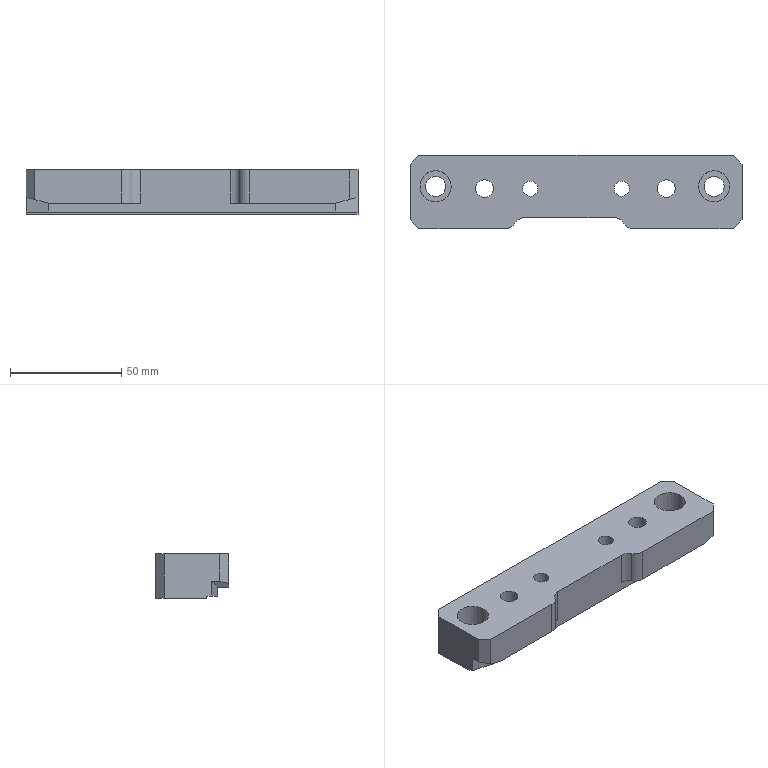Part | NX | features 20 2 | 1 solid | 34 faces | box 149 x 33 x 20 mm | volume 81598 mm3 | plane 22 | cylinder 12 | commonest cylinder face diameters 10 x4 6.8 x2 8.001 x2 9 x2 14 x2
STEP:
#1=CARTESIAN_POINT('',(540.502,427.372,-3.5));
#2=VERTEX_POINT('',#1);
#3=CARTESIAN_POINT('',(540.502,427.372,-2.5));
#4=VERTEX_POINT('',#3);
#5=CARTESIAN_POINT('',(540.502,427.372,11.5));
#6=DIRECTION('',(0.,0.,1.));
#7=VECTOR('',#6,1000.);
#8=LINE('',#5,#7);
#9=EDGE_CURVE('',#2,#4,#8,.T.);
#10=ORIENTED_EDGE('',*,*,#9,.F.);
#11=CARTESIAN_POINT('',(540.502,446.5,-3.5));
#12=VERTEX_POINT('',#11);
#13=CARTESIAN_POINT('',(540.502,450.5,-3.5));
#14=DIRECTION('',(0.,1.,0.));
#15=VECTOR('',#14,1000.);
#16=LINE('',#13,#15);
#17=EDGE_CURVE('',#2,#12,#16,.T.);
#18=ORIENTED_EDGE('',*,*,#17,.T.);
#19=CARTESIAN_POINT('',(540.502,446.5,16.5));
#20=VERTEX_POINT('',#19);
#21=CARTESIAN_POINT('',(540.502,446.5,11.5));
#22=DIRECTION('',(0.,0.,1.));
#23=VECTOR('',#22,1000.);
#24=LINE('',#21,#23);
#25=EDGE_CURVE('',#12,#20,#24,.T.);
#26=ORIENTED_EDGE('',*,*,#25,.T.);
#27=CARTESIAN_POINT('',(540.502,421.5,16.5));
#28=VERTEX_POINT('',#27);
#29=CARTESIAN_POINT('',(540.502,450.5,16.5));
#30=DIRECTION('',(0.,1.,0.));
#31=VECTOR('',#30,1000.);
#32=LINE('',#29,#31);
#33=EDGE_CURVE('',#28,#20,#32,.T.);
#34=ORIENTED_EDGE('',*,*,#33,.F.);
#35=CARTESIAN_POINT('',(540.502,421.5,4.179));
#36=VERTEX_POINT('',#35);
#37=CARTESIAN_POINT('',(540.502,421.5,11.5));
#38=DIRECTION('',(0.,0.,-1.));
#39=VECTOR('',#38,1000.);
#40=LINE('',#37,#39);
#41=EDGE_CURVE('',#28,#36,#40,.T.);
#42=ORIENTED_EDGE('',*,*,#41,.T.);
#43=CARTESIAN_POINT('',(540.502,425.18,4.179));
#44=VERTEX_POINT('',#43);
#45=CARTESIAN_POINT('',(540.502,417.5,4.179));
#46=DIRECTION('',(0.,1.,0.));
#47=VECTOR('',#46,1000.);
#48=LINE('',#45,#47);
#49=EDGE_CURVE('',#36,#44,#48,.T.);
#50=ORIENTED_EDGE('',*,*,#49,.T.);
#51=CARTESIAN_POINT('',(540.502,425.18,-2.5));
#52=VERTEX_POINT('',#51);
#53=CARTESIAN_POINT('',(540.502,425.18,3.5));
#54=DIRECTION('',(0.,0.,1.));
#55=VECTOR('',#54,1000.);
#56=LINE('',#53,#55);
#57=EDGE_CURVE('',#52,#44,#56,.T.);
#58=ORIENTED_EDGE('',*,*,#57,.F.);
#59=CARTESIAN_POINT('',(540.502,450.5,-2.5));
#60=DIRECTION('',(0.,1.,0.));
#61=VECTOR('',#60,1000.);
#62=LINE('',#59,#61);
#63=EDGE_CURVE('',#52,#4,#62,.T.);
#64=ORIENTED_EDGE('',*,*,#63,.T.);
#65=EDGE_LOOP('',(#10,#18,#26,#34,#42,#50,#58,#64));
#66=FACE_BOUND('',#65,.T.);
#67=CARTESIAN_POINT('',(540.502,450.5,11.5));
#68=DIRECTION('',(-1.,0.,0.));
#69=DIRECTION('',(0.,0.,-1.));
#70=AXIS2_PLACEMENT_3D('',#67,#68,#69);
#71=PLANE('',#70);
#72=ADVANCED_FACE('',(#66),#71,.F.);
#73=CARTESIAN_POINT('',(391.502,427.372,-2.5));
#74=VERTEX_POINT('',#73);
#75=CARTESIAN_POINT('',(391.502,427.372,-3.5));
#76=VERTEX_POINT('',#75);
#77=CARTESIAN_POINT('',(391.502,427.372,11.5));
#78=DIRECTION('',(0.,0.,-1.));
#79=VECTOR('',#78,1000.);
#80=LINE('',#77,#79);
#81=EDGE_CURVE('',#74,#76,#80,.T.);
#82=ORIENTED_EDGE('',*,*,#81,.F.);
#83=CARTESIAN_POINT('',(391.502,425.179,-2.5));
#84=VERTEX_POINT('',#83);
#85=CARTESIAN_POINT('',(391.502,417.5,-2.5));
#86=DIRECTION('',(0.,-1.,0.));
#87=VECTOR('',#86,1000.);
#88=LINE('',#85,#87);
#89=EDGE_CURVE('',#74,#84,#88,.T.);
#90=ORIENTED_EDGE('',*,*,#89,.T.);
#91=CARTESIAN_POINT('',(391.502,425.179,4.179));
#92=VERTEX_POINT('',#91);
#93=CARTESIAN_POINT('',(391.502,425.179,3.5));
#94=DIRECTION('',(0.,0.,1.));
#95=VECTOR('',#94,1000.);
#96=LINE('',#93,#95);
#97=EDGE_CURVE('',#84,#92,#96,.T.);
#98=ORIENTED_EDGE('',*,*,#97,.T.);
#99=CARTESIAN_POINT('',(391.502,421.5,4.179));
#100=VERTEX_POINT('',#99);
#101=CARTESIAN_POINT('',(391.502,425.179,4.179));
#102=DIRECTION('',(0.,-1.,0.));
#103=VECTOR('',#102,1000.);
#104=LINE('',#101,#103);
#105=EDGE_CURVE('',#92,#100,#104,.T.);
#106=ORIENTED_EDGE('',*,*,#105,.T.);
#107=CARTESIAN_POINT('',(391.502,421.5,16.5));
#108=VERTEX_POINT('',#107);
#109=CARTESIAN_POINT('',(391.502,421.5,11.5));
#110=DIRECTION('',(0.,0.,1.));
#111=VECTOR('',#110,1000.);
#112=LINE('',#109,#111);
#113=EDGE_CURVE('',#100,#108,#112,.T.);
#114=ORIENTED_EDGE('',*,*,#113,.T.);
#115=CARTESIAN_POINT('',(391.502,446.5,16.5));
#116=VERTEX_POINT('',#115);
#117=CARTESIAN_POINT('',(391.502,417.5,16.5));
#118=DIRECTION('',(0.,-1.,0.));
#119=VECTOR('',#118,1000.);
#120=LINE('',#117,#119);
#121=EDGE_CURVE('',#116,#108,#120,.T.);
#122=ORIENTED_EDGE('',*,*,#121,.F.);
#123=CARTESIAN_POINT('',(391.502,446.5,-3.5));
#124=VERTEX_POINT('',#123);
#125=CARTESIAN_POINT('',(391.502,446.5,11.5));
#126=DIRECTION('',(0.,0.,-1.));
#127=VECTOR('',#126,1000.);
#128=LINE('',#125,#127);
#129=EDGE_CURVE('',#116,#124,#128,.T.);
#130=ORIENTED_EDGE('',*,*,#129,.T.);
#131=CARTESIAN_POINT('',(391.502,417.5,-3.5));
#132=DIRECTION('',(0.,-1.,0.));
#133=VECTOR('',#132,1000.);
#134=LINE('',#131,#133);
#135=EDGE_CURVE('',#124,#76,#134,.T.);
#136=ORIENTED_EDGE('',*,*,#135,.T.);
#137=EDGE_LOOP('',(#82,#90,#98,#106,#114,#122,#130,#136));
#138=FACE_BOUND('',#137,.T.);
#139=CARTESIAN_POINT('',(391.502,417.5,11.5));
#140=DIRECTION('',(1.,0.,0.));
#141=DIRECTION('',(0.,0.,1.));
#142=AXIS2_PLACEMENT_3D('',#139,#140,#141);
#143=PLANE('',#142);
#144=ADVANCED_FACE('',(#138),#143,.F.);
#145=CARTESIAN_POINT('',(429.002,435.5,16.5));
#146=VERTEX_POINT('',#145);
#147=CARTESIAN_POINT('',(425.002,435.5,16.5));
#148=DIRECTION('',(0.,0.,1.));
#149=DIRECTION('',(1.,0.,0.));
#150=AXIS2_PLACEMENT_3D('',#147,#148,#149);
#151=CIRCLE('',#150,4.);
#152=EDGE_CURVE('',#146,#146,#151,.T.);
#153=ORIENTED_EDGE('',*,*,#152,.F.);
#154=EDGE_LOOP('',(#153));
#155=FACE_BOUND('',#154,.T.);
#156=CARTESIAN_POINT('',(510.502,435.5,16.5));
#157=VERTEX_POINT('',#156);
#158=CARTESIAN_POINT('',(506.502,435.5,16.5));
#159=DIRECTION('',(0.,0.,1.));
#160=DIRECTION('',(1.,0.,0.));
#161=AXIS2_PLACEMENT_3D('',#158,#159,#160);
#162=CIRCLE('',#161,4.);
#163=EDGE_CURVE('',#157,#157,#162,.T.);
#164=ORIENTED_EDGE('',*,*,#163,.F.);
#165=EDGE_LOOP('',(#164));
#166=FACE_BOUND('',#165,.T.);
#167=CARTESIAN_POINT('',(410.002,436.5,16.5));
#168=VERTEX_POINT('',#167);
#169=CARTESIAN_POINT('',(403.002,436.5,16.5));
#170=DIRECTION('',(0.,0.,1.));
#171=DIRECTION('',(1.,0.,0.));
#172=AXIS2_PLACEMENT_3D('',#169,#170,#171);
#173=CIRCLE('',#172,7.);
#174=EDGE_CURVE('',#168,#168,#173,.T.);
#175=ORIENTED_EDGE('',*,*,#174,.F.);
#176=EDGE_LOOP('',(#175));
#177=FACE_BOUND('',#176,.T.);
#178=CARTESIAN_POINT('',(535.002,436.5,16.5));
#179=VERTEX_POINT('',#178);
#180=CARTESIAN_POINT('',(528.002,436.5,16.5));
#181=DIRECTION('',(0.,0.,-1.));
#182=DIRECTION('',(1.,0.,0.));
#183=AXIS2_PLACEMENT_3D('',#180,#181,#182);
#184=CIRCLE('',#183,7.);
#185=EDGE_CURVE('',#179,#179,#184,.T.);
#186=ORIENTED_EDGE('',*,*,#185,.T.);
#187=EDGE_LOOP('',(#186));
#188=FACE_BOUND('',#187,.T.);
#189=ORIENTED_EDGE('',*,*,#121,.T.);
#190=CARTESIAN_POINT('',(395.502,417.5,16.5));
#191=VERTEX_POINT('',#190);
#192=CARTESIAN_POINT('',(391.502,421.5,16.5));
#193=DIRECTION('',(0.7071,-0.7071,0.));
#194=VECTOR('',#193,1000.);
#195=LINE('',#192,#194);
#196=EDGE_CURVE('',#108,#191,#195,.T.);
#197=ORIENTED_EDGE('',*,*,#196,.T.);
#198=CARTESIAN_POINT('',(434.268,417.5,16.5));
#199=VERTEX_POINT('',#198);
#200=CARTESIAN_POINT('',(368.002,417.5,16.5));
#201=DIRECTION('',(1.,0.,0.));
#202=VECTOR('',#201,1000.);
#203=LINE('',#200,#202);
#204=EDGE_CURVE('',#191,#199,#203,.T.);
#205=ORIENTED_EDGE('',*,*,#204,.T.);
#206=CARTESIAN_POINT('',(438.598,420.,16.5));
#207=VERTEX_POINT('',#206);
#208=CARTESIAN_POINT('',(434.268,422.5,16.5));
#209=DIRECTION('',(0.,0.,1.));
#210=DIRECTION('',(1.,0.,0.));
#211=AXIS2_PLACEMENT_3D('',#208,#209,#210);
#212=CIRCLE('',#211,5.);
#213=EDGE_CURVE('',#199,#207,#212,.T.);
#214=ORIENTED_EDGE('',*,*,#213,.T.);
#215=CARTESIAN_POINT('',(442.929,422.5,16.5));
#216=VERTEX_POINT('',#215);
#217=CARTESIAN_POINT('',(442.929,417.5,16.5));
#218=DIRECTION('',(0.,0.,1.));
#219=DIRECTION('',(1.,0.,0.));
#220=AXIS2_PLACEMENT_3D('',#217,#218,#219);
#221=CIRCLE('',#220,5.);
#222=EDGE_CURVE('',#216,#207,#221,.T.);
#223=ORIENTED_EDGE('',*,*,#222,.F.);
#224=CARTESIAN_POINT('',(483.129,422.5,16.5));
#225=VERTEX_POINT('',#224);
#226=CARTESIAN_POINT('',(368.002,422.5,16.5));
#227=DIRECTION('',(-1.,0.,0.));
#228=VECTOR('',#227,1000.);
#229=LINE('',#226,#228);
#230=EDGE_CURVE('',#225,#216,#229,.T.);
#231=ORIENTED_EDGE('',*,*,#230,.F.);
#232=CARTESIAN_POINT('',(487.459,420.,16.5));
#233=VERTEX_POINT('',#232);
#234=CARTESIAN_POINT('',(483.129,417.5,16.5));
#235=DIRECTION('',(0.,0.,1.));
#236=DIRECTION('',(1.,0.,0.));
#237=AXIS2_PLACEMENT_3D('',#234,#235,#236);
#238=CIRCLE('',#237,5.);
#239=EDGE_CURVE('',#233,#225,#238,.T.);
#240=ORIENTED_EDGE('',*,*,#239,.F.);
#241=CARTESIAN_POINT('',(491.789,417.5,16.5));
#242=VERTEX_POINT('',#241);
#243=CARTESIAN_POINT('',(491.789,422.5,16.5));
#244=DIRECTION('',(0.,0.,1.));
#245=DIRECTION('',(1.,0.,0.));
#246=AXIS2_PLACEMENT_3D('',#243,#244,#245);
#247=CIRCLE('',#246,5.);
#248=EDGE_CURVE('',#233,#242,#247,.T.);
#249=ORIENTED_EDGE('',*,*,#248,.T.);
#250=CARTESIAN_POINT('',(536.502,417.5,16.5));
#251=VERTEX_POINT('',#250);
#252=CARTESIAN_POINT('',(368.002,417.5,16.5));
#253=DIRECTION('',(1.,0.,0.));
#254=VECTOR('',#253,1000.);
#255=LINE('',#252,#254);
#256=EDGE_CURVE('',#242,#251,#255,.T.);
#257=ORIENTED_EDGE('',*,*,#256,.T.);
#258=CARTESIAN_POINT('',(536.502,417.5,16.5));
#259=DIRECTION('',(0.7071,0.7071,0.));
#260=VECTOR('',#259,1000.);
#261=LINE('',#258,#260);
#262=EDGE_CURVE('',#251,#28,#261,.T.);
#263=ORIENTED_EDGE('',*,*,#262,.T.);
#264=ORIENTED_EDGE('',*,*,#33,.T.);
#265=CARTESIAN_POINT('',(536.502,450.5,16.5));
#266=VERTEX_POINT('',#265);
#267=CARTESIAN_POINT('',(540.502,446.5,16.5));
#268=DIRECTION('',(-0.7071,0.7071,0.));
#269=VECTOR('',#268,1000.);
#270=LINE('',#267,#269);
#271=EDGE_CURVE('',#20,#266,#270,.T.);
#272=ORIENTED_EDGE('',*,*,#271,.T.);
#273=CARTESIAN_POINT('',(395.502,450.5,16.5));
#274=VERTEX_POINT('',#273);
#275=CARTESIAN_POINT('',(288.002,450.5,16.5));
#276=DIRECTION('',(-1.,0.,0.));
#277=VECTOR('',#276,1000.);
#278=LINE('',#275,#277);
#279=EDGE_CURVE('',#266,#274,#278,.T.);
#280=ORIENTED_EDGE('',*,*,#279,.T.);
#281=CARTESIAN_POINT('',(395.502,450.5,16.5));
#282=DIRECTION('',(-0.7071,-0.7071,0.));
#283=VECTOR('',#282,1000.);
#284=LINE('',#281,#283);
#285=EDGE_CURVE('',#274,#116,#284,.T.);
#286=ORIENTED_EDGE('',*,*,#285,.T.);
#287=EDGE_LOOP('',(#189,#197,#205,#214,#223,#231,#240,#249,#257,#263,#264,#272,#280,#286));
#288=FACE_BOUND('',#287,.T.);
#289=CARTESIAN_POINT('',(448.902,435.5,16.5));
#290=VERTEX_POINT('',#289);
#291=CARTESIAN_POINT('',(445.502,435.5,16.5));
#292=DIRECTION('',(0.,0.,-1.));
#293=DIRECTION('',(1.,0.,0.));
#294=AXIS2_PLACEMENT_3D('',#291,#292,#293);
#295=CIRCLE('',#294,3.4);
#296=EDGE_CURVE('',#290,#290,#295,.T.);
#297=ORIENTED_EDGE('',*,*,#296,.T.);
#298=EDGE_LOOP('',(#297));
#299=FACE_BOUND('',#298,.T.);
#300=CARTESIAN_POINT('',(489.902,435.5,16.5));
#301=VERTEX_POINT('',#300);
#302=CARTESIAN_POINT('',(486.502,435.5,16.5));
#303=DIRECTION('',(0.,0.,-1.));
#304=DIRECTION('',(1.,0.,0.));
#305=AXIS2_PLACEMENT_3D('',#302,#303,#304);
#306=CIRCLE('',#305,3.4);
#307=EDGE_CURVE('',#301,#301,#306,.T.);
#308=ORIENTED_EDGE('',*,*,#307,.T.);
#309=EDGE_LOOP('',(#308));
#310=FACE_BOUND('',#309,.T.);
#311=CARTESIAN_POINT('',(368.002,450.5,16.5));
#312=DIRECTION('',(0.,0.,1.));
#313=DIRECTION('',(-1.,0.,0.));
#314=AXIS2_PLACEMENT_3D('',#311,#312,#313);
#315=PLANE('',#314);
#316=ADVANCED_FACE('',(#155,#166,#177,#188,#288,#299,#310),#315,.T.);
#317=CARTESIAN_POINT('',(489.902,435.5,-3.5));
#318=VERTEX_POINT('',#317);
#319=CARTESIAN_POINT('',(486.502,435.5,-3.5));
#320=DIRECTION('',(0.,0.,-1.));
#321=DIRECTION('',(1.,0.,0.));
#322=AXIS2_PLACEMENT_3D('',#319,#320,#321);
#323=CIRCLE('',#322,3.4);
#324=EDGE_CURVE('',#318,#318,#323,.T.);
#325=ORIENTED_EDGE('',*,*,#324,.F.);
#326=EDGE_LOOP('',(#325));
#327=FACE_BOUND('',#326,.T.);
#328=CARTESIAN_POINT('',(398.502,436.5,-3.5));
#329=VERTEX_POINT('',#328);
#330=CARTESIAN_POINT('',(403.002,436.5,-3.5));
#331=DIRECTION('',(0.,0.,1.));
#332=DIRECTION('',(-1.,0.,0.));
#333=AXIS2_PLACEMENT_3D('',#330,#331,#332);
#334=CIRCLE('',#333,4.5);
#335=EDGE_CURVE('',#329,#329,#334,.T.);
#336=ORIENTED_EDGE('',*,*,#335,.T.);
#337=EDGE_LOOP('',(#336));
#338=FACE_BOUND('',#337,.T.);
#339=CARTESIAN_POINT('',(532.502,436.5,-3.5));
#340=VERTEX_POINT('',#339);
#341=CARTESIAN_POINT('',(528.002,436.5,-3.5));
#342=DIRECTION('',(0.,0.,1.));
#343=DIRECTION('',(1.,0.,0.));
#344=AXIS2_PLACEMENT_3D('',#341,#342,#343);
#345=CIRCLE('',#344,4.5);
#346=EDGE_CURVE('',#340,#340,#345,.T.);
#347=ORIENTED_EDGE('',*,*,#346,.T.);
#348=EDGE_LOOP('',(#347));
#349=FACE_BOUND('',#348,.T.);
#350=CARTESIAN_POINT('',(429.002,435.5,-3.5));
#351=VERTEX_POINT('',#350);
#352=CARTESIAN_POINT('',(425.002,435.5,-3.5));
#353=DIRECTION('',(0.,0.,-1.));
#354=DIRECTION('',(1.,0.,0.));
#355=AXIS2_PLACEMENT_3D('',#352,#353,#354);
#356=CIRCLE('',#355,4.);
#357=EDGE_CURVE('',#351,#351,#356,.T.);
#358=ORIENTED_EDGE('',*,*,#357,.F.);
#359=EDGE_LOOP('',(#358));
#360=FACE_BOUND('',#359,.T.);
#361=CARTESIAN_POINT('',(510.502,435.5,-3.5));
#362=VERTEX_POINT('',#361);
#363=CARTESIAN_POINT('',(506.502,435.5,-3.5));
#364=DIRECTION('',(0.,0.,1.));
#365=DIRECTION('',(1.,0.,0.));
#366=AXIS2_PLACEMENT_3D('',#363,#364,#365);
#367=CIRCLE('',#366,4.);
#368=EDGE_CURVE('',#362,#362,#367,.T.);
#369=ORIENTED_EDGE('',*,*,#368,.T.);
#370=EDGE_LOOP('',(#369));
#371=FACE_BOUND('',#370,.T.);
#372=CARTESIAN_POINT('',(448.902,435.5,-3.5));
#373=VERTEX_POINT('',#372);
#374=CARTESIAN_POINT('',(445.502,435.5,-3.5));
#375=DIRECTION('',(0.,0.,-1.));
#376=DIRECTION('',(1.,0.,0.));
#377=AXIS2_PLACEMENT_3D('',#374,#375,#376);
#378=CIRCLE('',#377,3.4);
#379=EDGE_CURVE('',#373,#373,#378,.T.);
#380=ORIENTED_EDGE('',*,*,#379,.F.);
#381=EDGE_LOOP('',(#380));
#382=FACE_BOUND('',#381,.T.);
#383=CARTESIAN_POINT('',(368.002,427.372,-3.5));
#384=DIRECTION('',(-1.,0.,0.));
#385=VECTOR('',#384,1000.);
#386=LINE('',#383,#385);
#387=EDGE_CURVE('',#2,#76,#386,.T.);
#388=ORIENTED_EDGE('',*,*,#387,.T.);
#389=ORIENTED_EDGE('',*,*,#135,.F.);
#390=CARTESIAN_POINT('',(395.502,450.5,-3.5));
#391=VERTEX_POINT('',#390);
#392=CARTESIAN_POINT('',(395.502,450.5,-3.5));
#393=DIRECTION('',(0.7071,0.7071,0.));
#394=VECTOR('',#393,1000.);
#395=LINE('',#392,#394);
#396=EDGE_CURVE('',#124,#391,#395,.T.);
#397=ORIENTED_EDGE('',*,*,#396,.T.);
#398=CARTESIAN_POINT('',(536.502,450.5,-3.5));
#399=VERTEX_POINT('',#398);
#400=CARTESIAN_POINT('',(288.002,450.5,-3.5));
#401=DIRECTION('',(-1.,0.,0.));
#402=VECTOR('',#401,1000.);
#403=LINE('',#400,#402);
#404=EDGE_CURVE('',#399,#391,#403,.T.);
#405=ORIENTED_EDGE('',*,*,#404,.F.);
#406=CARTESIAN_POINT('',(540.502,446.5,-3.5));
#407=DIRECTION('',(0.7071,-0.7071,0.));
#408=VECTOR('',#407,1000.);
#409=LINE('',#406,#408);
#410=EDGE_CURVE('',#399,#12,#409,.T.);
#411=ORIENTED_EDGE('',*,*,#410,.T.);
#412=ORIENTED_EDGE('',*,*,#17,.F.);
#413=EDGE_LOOP('',(#388,#389,#397,#405,#411,#412));
#414=FACE_BOUND('',#413,.T.);
#415=CARTESIAN_POINT('',(368.002,450.5,-3.5));
#416=DIRECTION('',(0.,0.,1.));
#417=DIRECTION('',(-1.,0.,0.));
#418=AXIS2_PLACEMENT_3D('',#415,#416,#417);
#419=PLANE('',#418);
#420=ADVANCED_FACE('',(#327,#338,#349,#360,#371,#382,#414),#419,.F.);
#421=ORIENTED_EDGE('',*,*,#357,.T.);
#422=EDGE_LOOP('',(#421));
#423=FACE_BOUND('',#422,.T.);
#424=ORIENTED_EDGE('',*,*,#152,.T.);
#425=EDGE_LOOP('',(#424));
#426=FACE_BOUND('',#425,.T.);
#427=CARTESIAN_POINT('',(425.002,435.5,42.5));
#428=DIRECTION('',(0.,0.,-1.));
#429=DIRECTION('',(1.,0.,0.));
#430=AXIS2_PLACEMENT_3D('',#427,#428,#429);
#431=CYLINDRICAL_SURFACE('',#430,4.);
#432=ADVANCED_FACE('',(#423,#426),#431,.F.);
#433=ORIENTED_EDGE('',*,*,#368,.F.);
#434=EDGE_LOOP('',(#433));
#435=FACE_BOUND('',#434,.T.);
#436=ORIENTED_EDGE('',*,*,#163,.T.);
#437=EDGE_LOOP('',(#436));
#438=FACE_BOUND('',#437,.T.);
#439=CARTESIAN_POINT('',(506.502,435.5,42.5));
#440=DIRECTION('',(0.,0.,-1.));
#441=DIRECTION('',(1.,0.,0.));
#442=AXIS2_PLACEMENT_3D('',#439,#440,#441);
#443=CYLINDRICAL_SURFACE('',#442,4.);
#444=ADVANCED_FACE('',(#435,#438),#443,.F.);
#445=ORIENTED_EDGE('',*,*,#174,.T.);
#446=EDGE_LOOP('',(#445));
#447=FACE_BOUND('',#446,.T.);
#448=CARTESIAN_POINT('',(410.002,436.5,6.5));
#449=VERTEX_POINT('',#448);
#450=CARTESIAN_POINT('',(403.002,436.5,6.5));
#451=DIRECTION('',(0.,0.,1.));
#452=DIRECTION('',(1.,0.,0.));
#453=AXIS2_PLACEMENT_3D('',#450,#451,#452);
#454=CIRCLE('',#453,7.);
#455=EDGE_CURVE('',#449,#449,#454,.T.);
#456=ORIENTED_EDGE('',*,*,#455,.F.);
#457=EDGE_LOOP('',(#456));
#458=FACE_BOUND('',#457,.T.);
#459=CARTESIAN_POINT('',(403.002,436.5,11.5));
#460=DIRECTION('',(0.,0.,-1.));
#461=DIRECTION('',(-1.,0.,0.));
#462=AXIS2_PLACEMENT_3D('',#459,#460,#461);
#463=CYLINDRICAL_SURFACE('',#462,7.);
#464=ADVANCED_FACE('',(#447,#458),#463,.F.);
#465=ORIENTED_EDGE('',*,*,#185,.F.);
#466=EDGE_LOOP('',(#465));
#467=FACE_BOUND('',#466,.T.);
#468=CARTESIAN_POINT('',(535.002,436.5,6.5));
#469=VERTEX_POINT('',#468);
#470=CARTESIAN_POINT('',(528.002,436.5,6.5));
#471=DIRECTION('',(0.,0.,1.));
#472=DIRECTION('',(1.,0.,0.));
#473=AXIS2_PLACEMENT_3D('',#470,#471,#472);
#474=CIRCLE('',#473,7.);
#475=EDGE_CURVE('',#469,#469,#474,.T.);
#476=ORIENTED_EDGE('',*,*,#475,.F.);
#477=EDGE_LOOP('',(#476));
#478=FACE_BOUND('',#477,.T.);
#479=CARTESIAN_POINT('',(528.002,436.5,11.5));
#480=DIRECTION('',(0.,0.,-1.));
#481=DIRECTION('',(-1.,0.,0.));
#482=AXIS2_PLACEMENT_3D('',#479,#480,#481);
#483=CYLINDRICAL_SURFACE('',#482,7.);
#484=ADVANCED_FACE('',(#467,#478),#483,.F.);
#485=ORIENTED_EDGE('',*,*,#25,.F.);
#486=ORIENTED_EDGE('',*,*,#410,.F.);
#487=CARTESIAN_POINT('',(536.502,450.5,11.5));
#488=DIRECTION('',(0.,0.,-1.));
#489=VECTOR('',#488,1000.);
#490=LINE('',#487,#489);
#491=EDGE_CURVE('',#266,#399,#490,.T.);
#492=ORIENTED_EDGE('',*,*,#491,.F.);
#493=ORIENTED_EDGE('',*,*,#271,.F.);
#494=EDGE_LOOP('',(#485,#486,#492,#493));
#495=FACE_BOUND('',#494,.T.);
#496=CARTESIAN_POINT('',(540.502,446.5,11.5));
#497=DIRECTION('',(-0.7071,-0.7071,0.));
#498=DIRECTION('',(0.,0.,-1.));
#499=AXIS2_PLACEMENT_3D('',#496,#497,#498);
#500=PLANE('',#499);
#501=ADVANCED_FACE('',(#495),#500,.F.);
#502=ORIENTED_EDGE('',*,*,#491,.T.);
#503=ORIENTED_EDGE('',*,*,#404,.T.);
#504=CARTESIAN_POINT('',(395.502,450.5,11.5));
#505=DIRECTION('',(0.,0.,1.));
#506=VECTOR('',#505,1000.);
#507=LINE('',#504,#506);
#508=EDGE_CURVE('',#391,#274,#507,.T.);
#509=ORIENTED_EDGE('',*,*,#508,.T.);
#510=ORIENTED_EDGE('',*,*,#279,.F.);
#511=EDGE_LOOP('',(#502,#503,#509,#510));
#512=FACE_BOUND('',#511,.T.);
#513=CARTESIAN_POINT('',(288.002,450.5,11.5));
#514=DIRECTION('',(0.,-1.,0.));
#515=DIRECTION('',(0.,0.,-1.));
#516=AXIS2_PLACEMENT_3D('',#513,#514,#515);
#517=PLANE('',#516);
#518=ADVANCED_FACE('',(#512),#517,.F.);
#519=ORIENTED_EDGE('',*,*,#508,.F.);
#520=ORIENTED_EDGE('',*,*,#396,.F.);
#521=ORIENTED_EDGE('',*,*,#129,.F.);
#522=ORIENTED_EDGE('',*,*,#285,.F.);
#523=EDGE_LOOP('',(#519,#520,#521,#522));
#524=FACE_BOUND('',#523,.T.);
#525=CARTESIAN_POINT('',(395.502,450.5,11.5));
#526=DIRECTION('',(0.7071,-0.7071,0.));
#527=DIRECTION('',(0.,0.,-1.));
#528=AXIS2_PLACEMENT_3D('',#525,#526,#527);
#529=PLANE('',#528);
#530=ADVANCED_FACE('',(#524),#529,.F.);
#531=CARTESIAN_POINT('',(407.502,436.5,6.5));
#532=VERTEX_POINT('',#531);
#533=CARTESIAN_POINT('',(403.002,436.5,6.5));
#534=DIRECTION('',(0.,0.,1.));
#535=DIRECTION('',(1.,0.,0.));
#536=AXIS2_PLACEMENT_3D('',#533,#534,#535);
#537=CIRCLE('',#536,4.5);
#538=EDGE_CURVE('',#532,#532,#537,.T.);
#539=ORIENTED_EDGE('',*,*,#538,.F.);
#540=EDGE_LOOP('',(#539));
#541=FACE_BOUND('',#540,.T.);
#542=ORIENTED_EDGE('',*,*,#455,.T.);
#543=EDGE_LOOP('',(#542));
#544=FACE_BOUND('',#543,.T.);
#545=CARTESIAN_POINT('',(542.502,302.3,6.5));
#546=DIRECTION('',(0.,0.,1.));
#547=DIRECTION('',(0.,1.,0.));
#548=AXIS2_PLACEMENT_3D('',#545,#546,#547);
#549=PLANE('',#548);
#550=ADVANCED_FACE('',(#541,#544),#549,.T.);
#551=ORIENTED_EDGE('',*,*,#538,.T.);
#552=EDGE_LOOP('',(#551));
#553=FACE_BOUND('',#552,.T.);
#554=ORIENTED_EDGE('',*,*,#335,.F.);
#555=EDGE_LOOP('',(#554));
#556=FACE_BOUND('',#555,.T.);
#557=CARTESIAN_POINT('',(403.002,436.5,-18.5));
#558=DIRECTION('',(0.,0.,-1.));
#559=DIRECTION('',(-1.,0.,0.));
#560=AXIS2_PLACEMENT_3D('',#557,#558,#559);
#561=CYLINDRICAL_SURFACE('',#560,4.5);
#562=ADVANCED_FACE('',(#553,#556),#561,.F.);
#563=CARTESIAN_POINT('',(532.502,436.5,6.5));
#564=VERTEX_POINT('',#563);
#565=CARTESIAN_POINT('',(528.002,436.5,6.5));
#566=DIRECTION('',(0.,0.,1.));
#567=DIRECTION('',(1.,0.,0.));
#568=AXIS2_PLACEMENT_3D('',#565,#566,#567);
#569=CIRCLE('',#568,4.5);
#570=EDGE_CURVE('',#564,#564,#569,.T.);
#571=ORIENTED_EDGE('',*,*,#570,.F.);
#572=EDGE_LOOP('',(#571));
#573=FACE_BOUND('',#572,.T.);
#574=ORIENTED_EDGE('',*,*,#475,.T.);
#575=EDGE_LOOP('',(#574));
#576=FACE_BOUND('',#575,.T.);
#577=CARTESIAN_POINT('',(667.502,302.3,6.5));
#578=DIRECTION('',(0.,0.,1.));
#579=DIRECTION('',(0.,1.,0.));
#580=AXIS2_PLACEMENT_3D('',#577,#578,#579);
#581=PLANE('',#580);
#582=ADVANCED_FACE('',(#573,#576),#581,.T.);
#583=ORIENTED_EDGE('',*,*,#570,.T.);
#584=EDGE_LOOP('',(#583));
#585=FACE_BOUND('',#584,.T.);
#586=ORIENTED_EDGE('',*,*,#346,.F.);
#587=EDGE_LOOP('',(#586));
#588=FACE_BOUND('',#587,.T.);
#589=CARTESIAN_POINT('',(528.002,436.5,-18.5));
#590=DIRECTION('',(0.,0.,-1.));
#591=DIRECTION('',(-1.,0.,0.));
#592=AXIS2_PLACEMENT_3D('',#589,#590,#591);
#593=CYLINDRICAL_SURFACE('',#592,4.5);
#594=ADVANCED_FACE('',(#585,#588),#593,.F.);
#595=ORIENTED_EDGE('',*,*,#296,.F.);
#596=EDGE_LOOP('',(#595));
#597=FACE_BOUND('',#596,.T.);
#598=ORIENTED_EDGE('',*,*,#379,.T.);
#599=EDGE_LOOP('',(#598));
#600=FACE_BOUND('',#599,.T.);
#601=CARTESIAN_POINT('',(445.502,435.5,-671.5));
#602=DIRECTION('',(0.,0.,1.));
#603=DIRECTION('',(-1.,0.,0.));
#604=AXIS2_PLACEMENT_3D('',#601,#602,#603);
#605=CYLINDRICAL_SURFACE('',#604,3.4);
#606=ADVANCED_FACE('',(#597,#600),#605,.F.);
#607=ORIENTED_EDGE('',*,*,#307,.F.);
#608=EDGE_LOOP('',(#607));
#609=FACE_BOUND('',#608,.T.);
#610=ORIENTED_EDGE('',*,*,#324,.T.);
#611=EDGE_LOOP('',(#610));
#612=FACE_BOUND('',#611,.T.);
#613=CARTESIAN_POINT('',(486.502,435.5,-671.5));
#614=DIRECTION('',(0.,0.,1.));
#615=DIRECTION('',(1.,0.,0.));
#616=AXIS2_PLACEMENT_3D('',#613,#614,#615);
#617=CYLINDRICAL_SURFACE('',#616,3.4);
#618=ADVANCED_FACE('',(#609,#612),#617,.F.);
#619=CARTESIAN_POINT('',(368.002,427.372,-2.5));
#620=DIRECTION('',(1.,0.,0.));
#621=VECTOR('',#620,1000.);
#622=LINE('',#619,#621);
#623=EDGE_CURVE('',#74,#4,#622,.T.);
#624=ORIENTED_EDGE('',*,*,#623,.F.);
#625=ORIENTED_EDGE('',*,*,#81,.T.);
#626=ORIENTED_EDGE('',*,*,#387,.F.);
#627=ORIENTED_EDGE('',*,*,#9,.T.);
#628=EDGE_LOOP('',(#624,#625,#626,#627));
#629=FACE_BOUND('',#628,.T.);
#630=CARTESIAN_POINT('',(496.583,427.372,-21.));
#631=DIRECTION('',(0.,-1.,0.));
#632=DIRECTION('',(0.,0.,1.));
#633=AXIS2_PLACEMENT_3D('',#630,#631,#632);
#634=PLANE('',#633);
#635=ADVANCED_FACE('',(#629),#634,.T.);
#636=CARTESIAN_POINT('',(438.598,420.,1.5));
#637=VERTEX_POINT('',#636);
#638=CARTESIAN_POINT('',(442.929,422.5,1.5));
#639=VERTEX_POINT('',#638);
#640=CARTESIAN_POINT('',(442.929,417.5,1.5));
#641=DIRECTION('',(0.,0.,-1.));
#642=DIRECTION('',(-1.,0.,0.));
#643=AXIS2_PLACEMENT_3D('',#640,#641,#642);
#644=CIRCLE('',#643,5.);
#645=EDGE_CURVE('',#637,#639,#644,.T.);
#646=ORIENTED_EDGE('',*,*,#645,.F.);
#647=CARTESIAN_POINT('',(434.268,417.5,1.5));
#648=VERTEX_POINT('',#647);
#649=CARTESIAN_POINT('',(434.268,422.5,1.5));
#650=DIRECTION('',(0.,0.,-1.));
#651=DIRECTION('',(-1.,0.,0.));
#652=AXIS2_PLACEMENT_3D('',#649,#650,#651);
#653=CIRCLE('',#652,5.);
#654=EDGE_CURVE('',#637,#648,#653,.T.);
#655=ORIENTED_EDGE('',*,*,#654,.T.);
#656=CARTESIAN_POINT('',(401.502,417.5,1.5));
#657=VERTEX_POINT('',#656);
#658=CARTESIAN_POINT('',(368.002,417.5,1.5));
#659=DIRECTION('',(-1.,0.,0.));
#660=VECTOR('',#659,1000.);
#661=LINE('',#658,#660);
#662=EDGE_CURVE('',#648,#657,#661,.T.);
#663=ORIENTED_EDGE('',*,*,#662,.T.);
#664=CARTESIAN_POINT('',(401.502,422.5,1.5));
#665=VERTEX_POINT('',#664);
#666=CARTESIAN_POINT('',(401.502,417.5,1.5));
#667=DIRECTION('',(0.,1.,0.));
#668=VECTOR('',#667,1000.);
#669=LINE('',#666,#668);
#670=EDGE_CURVE('',#657,#665,#669,.T.);
#671=ORIENTED_EDGE('',*,*,#670,.T.);
#672=CARTESIAN_POINT('',(358.,422.5,1.5));
#673=DIRECTION('',(-1.,0.,0.));
#674=VECTOR('',#673,1000.);
#675=LINE('',#672,#674);
#676=EDGE_CURVE('',#639,#665,#675,.T.);
#677=ORIENTED_EDGE('',*,*,#676,.F.);
#678=EDGE_LOOP('',(#646,#655,#663,#671,#677));
#679=FACE_BOUND('',#678,.T.);
#680=CARTESIAN_POINT('',(390.272,396.891,1.5));
#681=DIRECTION('',(0.,0.,-1.));
#682=DIRECTION('',(1.,0.,0.));
#683=AXIS2_PLACEMENT_3D('',#680,#681,#682);
#684=PLANE('',#683);
#685=ADVANCED_FACE('',(#679),#684,.T.);
#686=CARTESIAN_POINT('',(530.502,417.5,1.5));
#687=VERTEX_POINT('',#686);
#688=CARTESIAN_POINT('',(491.789,417.5,1.5));
#689=VERTEX_POINT('',#688);
#690=CARTESIAN_POINT('',(368.002,417.5,1.5));
#691=DIRECTION('',(-1.,0.,0.));
#692=VECTOR('',#691,1000.);
#693=LINE('',#690,#692);
#694=EDGE_CURVE('',#687,#689,#693,.T.);
#695=ORIENTED_EDGE('',*,*,#694,.T.);
#696=CARTESIAN_POINT('',(487.459,420.,1.5));
#697=VERTEX_POINT('',#696);
#698=CARTESIAN_POINT('',(491.789,422.5,1.5));
#699=DIRECTION('',(0.,0.,-1.));
#700=DIRECTION('',(-1.,0.,0.));
#701=AXIS2_PLACEMENT_3D('',#698,#699,#700);
#702=CIRCLE('',#701,5.);
#703=EDGE_CURVE('',#689,#697,#702,.T.);
#704=ORIENTED_EDGE('',*,*,#703,.T.);
#705=CARTESIAN_POINT('',(483.129,422.5,1.5));
#706=VERTEX_POINT('',#705);
#707=CARTESIAN_POINT('',(483.129,417.5,1.5));
#708=DIRECTION('',(0.,0.,-1.));
#709=DIRECTION('',(-1.,0.,0.));
#710=AXIS2_PLACEMENT_3D('',#707,#708,#709);
#711=CIRCLE('',#710,5.);
#712=EDGE_CURVE('',#706,#697,#711,.T.);
#713=ORIENTED_EDGE('',*,*,#712,.F.);
#714=CARTESIAN_POINT('',(530.5,422.5,1.5));
#715=VERTEX_POINT('',#714);
#716=CARTESIAN_POINT('',(358.,422.5,1.5));
#717=DIRECTION('',(-1.,0.,0.));
#718=VECTOR('',#717,1000.);
#719=LINE('',#716,#718);
#720=EDGE_CURVE('',#715,#706,#719,.T.);
#721=ORIENTED_EDGE('',*,*,#720,.F.);
#722=CARTESIAN_POINT('',(530.502,422.5,1.5));
#723=VERTEX_POINT('',#722);
#724=CARTESIAN_POINT('',(540.502,425.18,1.5));
#725=DIRECTION('',(-0.9659,-0.2588,0.));
#726=VECTOR('',#725,1000.);
#727=LINE('',#724,#726);
#728=EDGE_CURVE('',#723,#715,#727,.T.);
#729=ORIENTED_EDGE('',*,*,#728,.F.);
#730=CARTESIAN_POINT('',(530.502,425.18,1.5));
#731=DIRECTION('',(0.,-1.,0.));
#732=VECTOR('',#731,1000.);
#733=LINE('',#730,#732);
#734=EDGE_CURVE('',#723,#687,#733,.T.);
#735=ORIENTED_EDGE('',*,*,#734,.T.);
#736=EDGE_LOOP('',(#695,#704,#713,#721,#729,#735));
#737=FACE_BOUND('',#736,.T.);
#738=CARTESIAN_POINT('',(390.272,396.891,1.5));
#739=DIRECTION('',(0.,0.,-1.));
#740=DIRECTION('',(1.,0.,0.));
#741=AXIS2_PLACEMENT_3D('',#738,#739,#740);
#742=PLANE('',#741);
#743=ADVANCED_FACE('',(#737),#742,.T.);
#744=CARTESIAN_POINT('',(536.502,417.5,3.108));
#745=VERTEX_POINT('',#744);
#746=CARTESIAN_POINT('',(530.502,417.5,1.5));
#747=DIRECTION('',(0.9659,0.,0.2588));
#748=VECTOR('',#747,1000.);
#749=LINE('',#746,#748);
#750=EDGE_CURVE('',#687,#745,#749,.T.);
#751=ORIENTED_EDGE('',*,*,#750,.F.);
#752=ORIENTED_EDGE('',*,*,#734,.F.);
#753=CARTESIAN_POINT('',(539.874,425.012,4.011));
#754=DIRECTION('',(-0.9351,-0.2506,-0.2506));
#755=VECTOR('',#754,1000.);
#756=LINE('',#753,#755);
#757=EDGE_CURVE('',#44,#723,#756,.T.);
#758=ORIENTED_EDGE('',*,*,#757,.F.);
#759=ORIENTED_EDGE('',*,*,#49,.F.);
#760=CARTESIAN_POINT('',(523.45,404.449,-0.3894));
#761=DIRECTION('',(-0.6947,-0.6947,-0.1862));
#762=VECTOR('',#761,1000.);
#763=LINE('',#760,#762);
#764=EDGE_CURVE('',#36,#745,#763,.T.);
#765=ORIENTED_EDGE('',*,*,#764,.T.);
#766=EDGE_LOOP('',(#751,#752,#758,#759,#765));
#767=FACE_BOUND('',#766,.T.);
#768=CARTESIAN_POINT('',(530.502,396.891,1.5));
#769=DIRECTION('',(0.2588,0.,-0.9659));
#770=DIRECTION('',(0.9659,0.,0.2588));
#771=AXIS2_PLACEMENT_3D('',#768,#769,#770);
#772=PLANE('',#771);
#773=ADVANCED_FACE('',(#767),#772,.T.);
#774=ORIENTED_EDGE('',*,*,#105,.F.);
#775=CARTESIAN_POINT('',(401.501,422.5,1.5));
#776=VERTEX_POINT('',#775);
#777=CARTESIAN_POINT('',(401.501,422.5,1.5));
#778=DIRECTION('',(-0.9351,0.2506,0.2506));
#779=VECTOR('',#778,1000.);
#780=LINE('',#777,#779);
#781=EDGE_CURVE('',#776,#92,#780,.T.);
#782=ORIENTED_EDGE('',*,*,#781,.F.);
#783=CARTESIAN_POINT('',(457.481,422.5,-13.5));
#784=DIRECTION('',(-0.9659,0.,0.2588));
#785=VECTOR('',#784,1000.);
#786=LINE('',#783,#785);
#787=EDGE_CURVE('',#665,#776,#786,.T.);
#788=ORIENTED_EDGE('',*,*,#787,.F.);
#789=ORIENTED_EDGE('',*,*,#670,.F.);
#790=CARTESIAN_POINT('',(395.502,417.5,3.108));
#791=VERTEX_POINT('',#790);
#792=CARTESIAN_POINT('',(401.502,417.5,1.5));
#793=DIRECTION('',(0.9659,0.,-0.2588));
#794=VECTOR('',#793,1000.);
#795=LINE('',#792,#794);
#796=EDGE_CURVE('',#791,#657,#795,.T.);
#797=ORIENTED_EDGE('',*,*,#796,.F.);
#798=CARTESIAN_POINT('',(408.553,404.449,-0.3894));
#799=DIRECTION('',(-0.6947,0.6947,0.1862));
#800=VECTOR('',#799,1000.);
#801=LINE('',#798,#800);
#802=EDGE_CURVE('',#791,#100,#801,.T.);
#803=ORIENTED_EDGE('',*,*,#802,.T.);
#804=EDGE_LOOP('',(#774,#782,#788,#789,#797,#803));
#805=FACE_BOUND('',#804,.T.);
#806=CARTESIAN_POINT('',(401.502,396.891,1.5));
#807=DIRECTION('',(-0.2588,0.,-0.9659));
#808=DIRECTION('',(0.9659,0.,-0.2588));
#809=AXIS2_PLACEMENT_3D('',#806,#807,#808);
#810=PLANE('',#809);
#811=ADVANCED_FACE('',(#805),#810,.T.);
#812=CARTESIAN_POINT('',(536.502,417.5,11.5));
#813=DIRECTION('',(0.,0.,1.));
#814=VECTOR('',#813,1000.);
#815=LINE('',#812,#814);
#816=EDGE_CURVE('',#745,#251,#815,.T.);
#817=ORIENTED_EDGE('',*,*,#816,.F.);
#818=ORIENTED_EDGE('',*,*,#764,.F.);
#819=ORIENTED_EDGE('',*,*,#41,.F.);
#820=ORIENTED_EDGE('',*,*,#262,.F.);
#821=EDGE_LOOP('',(#817,#818,#819,#820));
#822=FACE_BOUND('',#821,.T.);
#823=CARTESIAN_POINT('',(536.502,417.5,11.5));
#824=DIRECTION('',(-0.7071,0.7071,0.));
#825=DIRECTION('',(0.,0.,-1.));
#826=AXIS2_PLACEMENT_3D('',#823,#824,#825);
#827=PLANE('',#826);
#828=ADVANCED_FACE('',(#822),#827,.F.);
#829=ORIENTED_EDGE('',*,*,#256,.F.);
#830=CARTESIAN_POINT('',(491.789,417.5,11.5));
#831=DIRECTION('',(0.,0.,-1.));
#832=VECTOR('',#831,1000.);
#833=LINE('',#830,#832);
#834=EDGE_CURVE('',#242,#689,#833,.T.);
#835=ORIENTED_EDGE('',*,*,#834,.T.);
#836=ORIENTED_EDGE('',*,*,#694,.F.);
#837=ORIENTED_EDGE('',*,*,#750,.T.);
#838=ORIENTED_EDGE('',*,*,#816,.T.);
#839=EDGE_LOOP('',(#829,#835,#836,#837,#838));
#840=FACE_BOUND('',#839,.T.);
#841=CARTESIAN_POINT('',(368.002,417.5,11.5));
#842=DIRECTION('',(0.,1.,0.));
#843=DIRECTION('',(0.,0.,1.));
#844=AXIS2_PLACEMENT_3D('',#841,#842,#843);
#845=PLANE('',#844);
#846=ADVANCED_FACE('',(#840),#845,.F.);
#847=ORIENTED_EDGE('',*,*,#703,.F.);
#848=ORIENTED_EDGE('',*,*,#834,.F.);
#849=ORIENTED_EDGE('',*,*,#248,.F.);
#850=CARTESIAN_POINT('',(487.459,420.,-7.5));
#851=DIRECTION('',(0.,0.,1.));
#852=VECTOR('',#851,1000.);
#853=LINE('',#850,#852);
#854=EDGE_CURVE('',#697,#233,#853,.T.);
#855=ORIENTED_EDGE('',*,*,#854,.F.);
#856=EDGE_LOOP('',(#847,#848,#849,#855));
#857=FACE_BOUND('',#856,.T.);
#858=CARTESIAN_POINT('',(491.789,422.5,-7.5));
#859=DIRECTION('',(0.,0.,1.));
#860=DIRECTION('',(-1.,0.,0.));
#861=AXIS2_PLACEMENT_3D('',#858,#859,#860);
#862=CYLINDRICAL_SURFACE('',#861,5.);
#863=ADVANCED_FACE('',(#857),#862,.T.);
#864=ORIENTED_EDGE('',*,*,#712,.T.);
#865=ORIENTED_EDGE('',*,*,#854,.T.);
#866=ORIENTED_EDGE('',*,*,#239,.T.);
#867=CARTESIAN_POINT('',(483.129,422.5,3.5));
#868=DIRECTION('',(0.,0.,-1.));
#869=VECTOR('',#868,1000.);
#870=LINE('',#867,#869);
#871=EDGE_CURVE('',#225,#706,#870,.T.);
#872=ORIENTED_EDGE('',*,*,#871,.T.);
#873=EDGE_LOOP('',(#864,#865,#866,#872));
#874=FACE_BOUND('',#873,.T.);
#875=CARTESIAN_POINT('',(483.129,417.5,-7.5));
#876=DIRECTION('',(0.,0.,1.));
#877=DIRECTION('',(-1.,0.,0.));
#878=AXIS2_PLACEMENT_3D('',#875,#876,#877);
#879=CYLINDRICAL_SURFACE('',#878,5.);
#880=ADVANCED_FACE('',(#874),#879,.F.);
#881=ORIENTED_EDGE('',*,*,#222,.T.);
#882=CARTESIAN_POINT('',(438.598,420.,3.5));
#883=DIRECTION('',(0.,0.,-1.));
#884=VECTOR('',#883,1000.);
#885=LINE('',#882,#884);
#886=EDGE_CURVE('',#207,#637,#885,.T.);
#887=ORIENTED_EDGE('',*,*,#886,.T.);
#888=ORIENTED_EDGE('',*,*,#645,.T.);
#889=CARTESIAN_POINT('',(442.929,422.5,3.5));
#890=DIRECTION('',(0.,0.,1.));
#891=VECTOR('',#890,1000.);
#892=LINE('',#889,#891);
#893=EDGE_CURVE('',#639,#216,#892,.T.);
#894=ORIENTED_EDGE('',*,*,#893,.T.);
#895=EDGE_LOOP('',(#881,#887,#888,#894));
#896=FACE_BOUND('',#895,.T.);
#897=CARTESIAN_POINT('',(442.929,417.5,3.5));
#898=DIRECTION('',(0.,0.,1.));
#899=DIRECTION('',(-1.,0.,0.));
#900=AXIS2_PLACEMENT_3D('',#897,#898,#899);
#901=CYLINDRICAL_SURFACE('',#900,5.);
#902=ADVANCED_FACE('',(#896),#901,.F.);
#903=ORIENTED_EDGE('',*,*,#213,.F.);
#904=CARTESIAN_POINT('',(434.268,417.5,11.5));
#905=DIRECTION('',(0.,0.,1.));
#906=VECTOR('',#905,1000.);
#907=LINE('',#904,#906);
#908=EDGE_CURVE('',#648,#199,#907,.T.);
#909=ORIENTED_EDGE('',*,*,#908,.F.);
#910=ORIENTED_EDGE('',*,*,#654,.F.);
#911=ORIENTED_EDGE('',*,*,#886,.F.);
#912=EDGE_LOOP('',(#903,#909,#910,#911));
#913=FACE_BOUND('',#912,.T.);
#914=CARTESIAN_POINT('',(434.268,422.5,3.5));
#915=DIRECTION('',(0.,0.,1.));
#916=DIRECTION('',(-1.,0.,0.));
#917=AXIS2_PLACEMENT_3D('',#914,#915,#916);
#918=CYLINDRICAL_SURFACE('',#917,5.);
#919=ADVANCED_FACE('',(#913),#918,.T.);
#920=ORIENTED_EDGE('',*,*,#662,.F.);
#921=ORIENTED_EDGE('',*,*,#908,.T.);
#922=ORIENTED_EDGE('',*,*,#204,.F.);
#923=CARTESIAN_POINT('',(395.502,417.5,11.5));
#924=DIRECTION('',(0.,0.,-1.));
#925=VECTOR('',#924,1000.);
#926=LINE('',#923,#925);
#927=EDGE_CURVE('',#191,#791,#926,.T.);
#928=ORIENTED_EDGE('',*,*,#927,.T.);
#929=ORIENTED_EDGE('',*,*,#796,.T.);
#930=EDGE_LOOP('',(#920,#921,#922,#928,#929));
#931=FACE_BOUND('',#930,.T.);
#932=CARTESIAN_POINT('',(368.002,417.5,11.5));
#933=DIRECTION('',(0.,1.,0.));
#934=DIRECTION('',(0.,0.,1.));
#935=AXIS2_PLACEMENT_3D('',#932,#933,#934);
#936=PLANE('',#935);
#937=ADVANCED_FACE('',(#931),#936,.F.);
#938=ORIENTED_EDGE('',*,*,#113,.F.);
#939=ORIENTED_EDGE('',*,*,#802,.F.);
#940=ORIENTED_EDGE('',*,*,#927,.F.);
#941=ORIENTED_EDGE('',*,*,#196,.F.);
#942=EDGE_LOOP('',(#938,#939,#940,#941));
#943=FACE_BOUND('',#942,.T.);
#944=CARTESIAN_POINT('',(391.502,421.5,11.5));
#945=DIRECTION('',(0.7071,0.7071,0.));
#946=DIRECTION('',(0.,0.,-1.));
#947=AXIS2_PLACEMENT_3D('',#944,#945,#946);
#948=PLANE('',#947);
#949=ADVANCED_FACE('',(#943),#948,.F.);
#950=CARTESIAN_POINT('',(401.501,422.5,-2.5));
#951=VERTEX_POINT('',#950);
#952=CARTESIAN_POINT('',(401.501,422.5,-2.5));
#953=DIRECTION('',(0.9659,-0.2588,0.));
#954=VECTOR('',#953,1000.);
#955=LINE('',#952,#954);
#956=EDGE_CURVE('',#84,#951,#955,.T.);
#957=ORIENTED_EDGE('',*,*,#956,.T.);
#958=CARTESIAN_POINT('',(401.501,422.5,3.5));
#959=DIRECTION('',(0.,0.,-1.));
#960=VECTOR('',#959,1000.);
#961=LINE('',#958,#960);
#962=EDGE_CURVE('',#776,#951,#961,.T.);
#963=ORIENTED_EDGE('',*,*,#962,.F.);
#964=ORIENTED_EDGE('',*,*,#781,.T.);
#965=ORIENTED_EDGE('',*,*,#97,.F.);
#966=EDGE_LOOP('',(#957,#963,#964,#965));
#967=FACE_BOUND('',#966,.T.);
#968=CARTESIAN_POINT('',(401.501,422.5,3.5));
#969=DIRECTION('',(0.2588,0.9659,0.));
#970=DIRECTION('',(0.9659,-0.2588,0.));
#971=AXIS2_PLACEMENT_3D('',#968,#969,#970);
#972=PLANE('',#971);
#973=ADVANCED_FACE('',(#967),#972,.F.);
#974=ORIENTED_EDGE('',*,*,#720,.T.);
#975=ORIENTED_EDGE('',*,*,#871,.F.);
#976=ORIENTED_EDGE('',*,*,#230,.T.);
#977=ORIENTED_EDGE('',*,*,#893,.F.);
#978=ORIENTED_EDGE('',*,*,#676,.T.);
#979=ORIENTED_EDGE('',*,*,#787,.T.);
#980=ORIENTED_EDGE('',*,*,#962,.T.);
#981=CARTESIAN_POINT('',(530.5,422.5,-2.5));
#982=VERTEX_POINT('',#981);
#983=CARTESIAN_POINT('',(358.,422.5,-2.5));
#984=DIRECTION('',(1.,0.,0.));
#985=VECTOR('',#984,1000.);
#986=LINE('',#983,#985);
#987=EDGE_CURVE('',#951,#982,#986,.T.);
#988=ORIENTED_EDGE('',*,*,#987,.T.);
#989=CARTESIAN_POINT('',(530.5,422.5,3.5));
#990=DIRECTION('',(0.,0.,-1.));
#991=VECTOR('',#990,1000.);
#992=LINE('',#989,#991);
#993=EDGE_CURVE('',#715,#982,#992,.T.);
#994=ORIENTED_EDGE('',*,*,#993,.F.);
#995=EDGE_LOOP('',(#974,#975,#976,#977,#978,#979,#980,#988,#994));
#996=FACE_BOUND('',#995,.T.);
#997=CARTESIAN_POINT('',(358.,422.5,3.5));
#998=DIRECTION('',(0.,1.,0.));
#999=DIRECTION('',(0.,0.,1.));
#1000=AXIS2_PLACEMENT_3D('',#997,#998,#999);
#1001=PLANE('',#1000);
#1002=ADVANCED_FACE('',(#996),#1001,.F.);
#1003=CARTESIAN_POINT('',(540.502,425.18,-2.5));
#1004=DIRECTION('',(0.9659,0.2588,0.));
#1005=VECTOR('',#1004,1000.);
#1006=LINE('',#1003,#1005);
#1007=EDGE_CURVE('',#982,#52,#1006,.T.);
#1008=ORIENTED_EDGE('',*,*,#1007,.T.);
#1009=ORIENTED_EDGE('',*,*,#57,.T.);
#1010=ORIENTED_EDGE('',*,*,#757,.T.);
#1011=ORIENTED_EDGE('',*,*,#728,.T.);
#1012=ORIENTED_EDGE('',*,*,#993,.T.);
#1013=EDGE_LOOP('',(#1008,#1009,#1010,#1011,#1012));
#1014=FACE_BOUND('',#1013,.T.);
#1015=CARTESIAN_POINT('',(540.502,425.18,3.5));
#1016=DIRECTION('',(-0.2588,0.9659,0.));
#1017=DIRECTION('',(0.9659,0.2588,0.));
#1018=AXIS2_PLACEMENT_3D('',#1015,#1016,#1017);
#1019=PLANE('',#1018);
#1020=ADVANCED_FACE('',(#1014),#1019,.F.);
#1021=ORIENTED_EDGE('',*,*,#89,.F.);
#1022=ORIENTED_EDGE('',*,*,#623,.T.);
#1023=ORIENTED_EDGE('',*,*,#63,.F.);
#1024=ORIENTED_EDGE('',*,*,#1007,.F.);
#1025=ORIENTED_EDGE('',*,*,#987,.F.);
#1026=ORIENTED_EDGE('',*,*,#956,.F.);
#1027=EDGE_LOOP('',(#1021,#1022,#1023,#1024,#1025,#1026));
#1028=FACE_BOUND('',#1027,.T.);
#1029=CARTESIAN_POINT('',(368.002,450.5,-2.5));
#1030=DIRECTION('',(0.,0.,1.));
#1031=DIRECTION('',(-1.,0.,0.));
#1032=AXIS2_PLACEMENT_3D('',#1029,#1030,#1031);
#1033=PLANE('',#1032);
#1034=ADVANCED_FACE('',(#1028),#1033,.F.);
#1035=CLOSED_SHELL('',(#72,#144,#316,#420,#432,#444,#464,#484,#501,#518,#530,#550,#562,#582,#594,#606,#618,#635,#685,#743,#773,#811,#828,#846,#863,#880,#902,#919,#937,#949,#973,#1002,#1020,#1034));
#1036=MANIFOLD_SOLID_BREP('',#1035);
#1037=(LENGTH_UNIT()NAMED_UNIT(*)SI_UNIT(.MILLI.,.METRE.));
#1038=UNCERTAINTY_MEASURE_WITH_UNIT(LENGTH_MEASURE(0.00001),#1037,'','');
#1039=(NAMED_UNIT(*)PLANE_ANGLE_UNIT()SI_UNIT($,.RADIAN.));
#1040=(NAMED_UNIT(*)SI_UNIT($,.STERADIAN.)SOLID_ANGLE_UNIT());
#1041=(GEOMETRIC_REPRESENTATION_CONTEXT(3)GLOBAL_UNCERTAINTY_ASSIGNED_CONTEXT((#1038))GLOBAL_UNIT_ASSIGNED_CONTEXT((#1037,#1039,#1040))REPRESENTATION_CONTEXT('',''));
#1042=ADVANCED_BREP_SHAPE_REPRESENTATION('',(#1036),#1041);